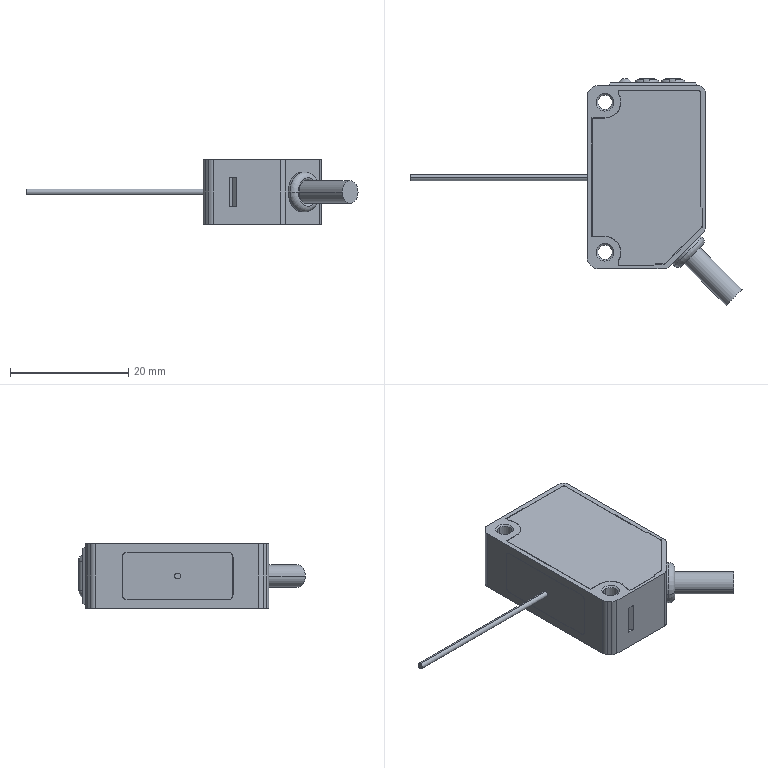Part | SolidWorks | features BaseBody 1, ICE 1 | 1 solid | 212 faces | box 56.19 x 38.39 x 11 mm | volume 6633 mm3 | plane 115 | cylinder 79 | torus 8 | cone 8 | sphere 2 | commonest cylinder face diameters 2 x9 4.02 x8 2.4 x7 2.3 x6 0.8 x4 1.6 x4